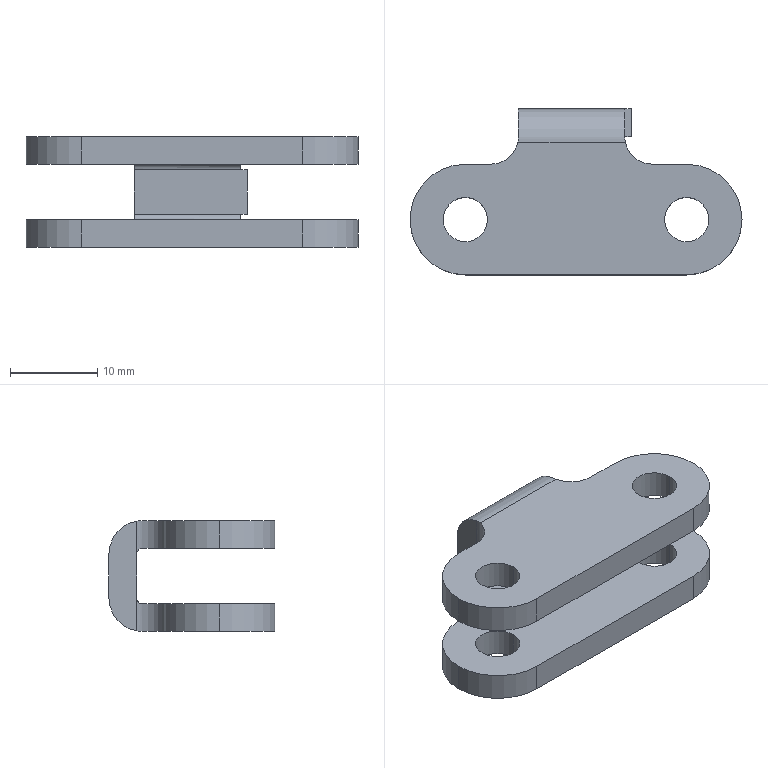Part | SolidWorks | features Cut 3, Fillet 3, Boss 1, Extrusion 1 | 1 solid | 42 faces | box 38.1 x 19.05 x 12.7 mm | volume 3299 mm3 | cylinder 24 | plane 18 | commonest cylinder face diameters 5.08 x8 12.7 x8 6.35 x4 1.27 x2 7.62 x2
STEP:
#1=CARTESIAN_POINT('',(0.9,0.,-0.5));
#2=VERTEX_POINT('',#1);
#3=CARTESIAN_POINT('',(1.1,0.,-0.5));
#4=VERTEX_POINT('',#3);
#5=CARTESIAN_POINT('',(1.,0.,-0.5));
#6=DIRECTION('',(0.,0.,1.));
#7=DIRECTION('',(1.,0.,0.));
#8=AXIS2_PLACEMENT_3D('',#5,#6,#7);
#9=CIRCLE('',#8,0.1);
#10=EDGE_CURVE('',#2,#4,#9,.T.);
#11=ORIENTED_EDGE('',*,*,#10,.F.);
#12=CARTESIAN_POINT('',(0.9,0.,-0.375));
#13=VERTEX_POINT('',#12);
#14=CARTESIAN_POINT('',(0.9,0.,-0.5));
#15=DIRECTION('',(0.,0.,1.));
#16=VECTOR('',#15,39.37);
#17=LINE('',#14,#16);
#18=EDGE_CURVE('',#2,#13,#17,.T.);
#19=ORIENTED_EDGE('',*,*,#18,.T.);
#20=CARTESIAN_POINT('',(1.1,0.,-0.375));
#21=VERTEX_POINT('',#20);
#22=CARTESIAN_POINT('',(1.,0.,-0.375));
#23=DIRECTION('',(0.,0.,1.));
#24=DIRECTION('',(0.,1.,0.));
#25=AXIS2_PLACEMENT_3D('',#22,#23,#24);
#26=CIRCLE('',#25,0.1);
#27=EDGE_CURVE('',#13,#21,#26,.T.);
#28=ORIENTED_EDGE('',*,*,#27,.T.);
#29=CARTESIAN_POINT('',(1.1,0.,-0.5));
#30=DIRECTION('',(0.,0.,1.));
#31=VECTOR('',#30,39.37);
#32=LINE('',#29,#31);
#33=EDGE_CURVE('',#4,#21,#32,.T.);
#34=ORIENTED_EDGE('',*,*,#33,.F.);
#35=EDGE_LOOP('',(#11,#19,#28,#34));
#36=FACE_OUTER_BOUND('',#35,.T.);
#37=CARTESIAN_POINT('',(1.,0.,-0.5));
#38=DIRECTION('',(0.,0.,1.));
#39=DIRECTION('',(1.,0.,0.));
#40=AXIS2_PLACEMENT_3D('',#37,#38,#39);
#41=CYLINDRICAL_SURFACE('',#40,0.1);
#42=ADVANCED_FACE('',(#36),#41,.F.);
#43=CARTESIAN_POINT('',(-0.1,0.,-0.5));
#44=VERTEX_POINT('',#43);
#45=CARTESIAN_POINT('',(0.1,0.,-0.5));
#46=VERTEX_POINT('',#45);
#47=CARTESIAN_POINT('',(0.,0.,-0.5));
#48=DIRECTION('',(0.,0.,1.));
#49=DIRECTION('',(1.,0.,0.));
#50=AXIS2_PLACEMENT_3D('',#47,#48,#49);
#51=CIRCLE('',#50,0.1);
#52=EDGE_CURVE('',#44,#46,#51,.T.);
#53=ORIENTED_EDGE('',*,*,#52,.F.);
#54=CARTESIAN_POINT('',(-0.1,0.,-0.375));
#55=VERTEX_POINT('',#54);
#56=CARTESIAN_POINT('',(-0.1,0.,-0.5));
#57=DIRECTION('',(0.,0.,1.));
#58=VECTOR('',#57,39.37);
#59=LINE('',#56,#58);
#60=EDGE_CURVE('',#44,#55,#59,.T.);
#61=ORIENTED_EDGE('',*,*,#60,.T.);
#62=CARTESIAN_POINT('',(0.1,0.,-0.375));
#63=VERTEX_POINT('',#62);
#64=CARTESIAN_POINT('',(0.,0.,-0.375));
#65=DIRECTION('',(0.,0.,1.));
#66=DIRECTION('',(0.,1.,0.));
#67=AXIS2_PLACEMENT_3D('',#64,#65,#66);
#68=CIRCLE('',#67,0.1);
#69=EDGE_CURVE('',#55,#63,#68,.T.);
#70=ORIENTED_EDGE('',*,*,#69,.T.);
#71=CARTESIAN_POINT('',(0.1,0.,-0.5));
#72=DIRECTION('',(0.,0.,1.));
#73=VECTOR('',#72,39.37);
#74=LINE('',#71,#73);
#75=EDGE_CURVE('',#46,#63,#74,.T.);
#76=ORIENTED_EDGE('',*,*,#75,.F.);
#77=EDGE_LOOP('',(#53,#61,#70,#76));
#78=FACE_OUTER_BOUND('',#77,.T.);
#79=CARTESIAN_POINT('',(0.,0.,-0.5));
#80=DIRECTION('',(0.,0.,1.));
#81=DIRECTION('',(1.,0.,0.));
#82=AXIS2_PLACEMENT_3D('',#79,#80,#81);
#83=CYLINDRICAL_SURFACE('',#82,0.1);
#84=ADVANCED_FACE('',(#78),#83,.F.);
#85=CARTESIAN_POINT('',(1.1,0.,-0.125));
#86=VERTEX_POINT('',#85);
#87=CARTESIAN_POINT('',(0.9,0.,-0.125));
#88=VERTEX_POINT('',#87);
#89=CARTESIAN_POINT('',(1.,0.,-0.125));
#90=DIRECTION('',(0.,0.,-1.));
#91=DIRECTION('',(0.,-1.,0.));
#92=AXIS2_PLACEMENT_3D('',#89,#90,#91);
#93=CIRCLE('',#92,0.1);
#94=EDGE_CURVE('',#86,#88,#93,.T.);
#95=ORIENTED_EDGE('',*,*,#94,.T.);
#96=CARTESIAN_POINT('',(0.9,0.,0.));
#97=VERTEX_POINT('',#96);
#98=CARTESIAN_POINT('',(0.9,0.,-0.5));
#99=DIRECTION('',(0.,0.,1.));
#100=VECTOR('',#99,39.37);
#101=LINE('',#98,#100);
#102=EDGE_CURVE('',#88,#97,#101,.T.);
#103=ORIENTED_EDGE('',*,*,#102,.T.);
#104=CARTESIAN_POINT('',(1.1,0.,0.));
#105=VERTEX_POINT('',#104);
#106=CARTESIAN_POINT('',(1.,0.,0.));
#107=DIRECTION('',(0.,0.,1.));
#108=DIRECTION('',(1.,0.,0.));
#109=AXIS2_PLACEMENT_3D('',#106,#107,#108);
#110=CIRCLE('',#109,0.1);
#111=EDGE_CURVE('',#97,#105,#110,.T.);
#112=ORIENTED_EDGE('',*,*,#111,.T.);
#113=CARTESIAN_POINT('',(1.1,0.,-0.5));
#114=DIRECTION('',(0.,0.,1.));
#115=VECTOR('',#114,39.37);
#116=LINE('',#113,#115);
#117=EDGE_CURVE('',#86,#105,#116,.T.);
#118=ORIENTED_EDGE('',*,*,#117,.F.);
#119=EDGE_LOOP('',(#95,#103,#112,#118));
#120=FACE_OUTER_BOUND('',#119,.T.);
#121=CARTESIAN_POINT('',(1.,0.,-0.5));
#122=DIRECTION('',(0.,0.,1.));
#123=DIRECTION('',(1.,0.,0.));
#124=AXIS2_PLACEMENT_3D('',#121,#122,#123);
#125=CYLINDRICAL_SURFACE('',#124,0.1);
#126=ADVANCED_FACE('',(#120),#125,.F.);
#127=CARTESIAN_POINT('',(0.1,0.,-0.125));
#128=VERTEX_POINT('',#127);
#129=CARTESIAN_POINT('',(-0.1,0.,-0.125));
#130=VERTEX_POINT('',#129);
#131=CARTESIAN_POINT('',(0.,0.,-0.125));
#132=DIRECTION('',(0.,0.,-1.));
#133=DIRECTION('',(0.,-1.,0.));
#134=AXIS2_PLACEMENT_3D('',#131,#132,#133);
#135=CIRCLE('',#134,0.1);
#136=EDGE_CURVE('',#128,#130,#135,.T.);
#137=ORIENTED_EDGE('',*,*,#136,.T.);
#138=CARTESIAN_POINT('',(-0.1,0.,0.));
#139=VERTEX_POINT('',#138);
#140=CARTESIAN_POINT('',(-0.1,0.,-0.5));
#141=DIRECTION('',(0.,0.,1.));
#142=VECTOR('',#141,39.37);
#143=LINE('',#140,#142);
#144=EDGE_CURVE('',#130,#139,#143,.T.);
#145=ORIENTED_EDGE('',*,*,#144,.T.);
#146=CARTESIAN_POINT('',(0.1,0.,0.));
#147=VERTEX_POINT('',#146);
#148=CARTESIAN_POINT('',(0.,0.,0.));
#149=DIRECTION('',(0.,0.,1.));
#150=DIRECTION('',(1.,0.,0.));
#151=AXIS2_PLACEMENT_3D('',#148,#149,#150);
#152=CIRCLE('',#151,0.1);
#153=EDGE_CURVE('',#139,#147,#152,.T.);
#154=ORIENTED_EDGE('',*,*,#153,.T.);
#155=CARTESIAN_POINT('',(0.1,0.,-0.5));
#156=DIRECTION('',(0.,0.,1.));
#157=VECTOR('',#156,39.37);
#158=LINE('',#155,#157);
#159=EDGE_CURVE('',#128,#147,#158,.T.);
#160=ORIENTED_EDGE('',*,*,#159,.F.);
#161=EDGE_LOOP('',(#137,#145,#154,#160));
#162=FACE_OUTER_BOUND('',#161,.T.);
#163=CARTESIAN_POINT('',(0.,0.,-0.5));
#164=DIRECTION('',(0.,0.,1.));
#165=DIRECTION('',(1.,0.,0.));
#166=AXIS2_PLACEMENT_3D('',#163,#164,#165);
#167=CYLINDRICAL_SURFACE('',#166,0.1);
#168=ADVANCED_FACE('',(#162),#167,.F.);
#169=CARTESIAN_POINT('',(0.72,0.5,-0.15));
#170=VERTEX_POINT('',#169);
#171=CARTESIAN_POINT('',(0.72,0.375,-0.15));
#172=VERTEX_POINT('',#171);
#173=CARTESIAN_POINT('',(0.72,0.5,-0.15));
#174=DIRECTION('',(0.,-1.,0.));
#175=VECTOR('',#174,39.37);
#176=LINE('',#173,#175);
#177=EDGE_CURVE('',#170,#172,#176,.T.);
#178=ORIENTED_EDGE('',*,*,#177,.F.);
#179=CARTESIAN_POINT('',(0.72,0.375,-0.002098));
#180=VERTEX_POINT('',#179);
#181=CARTESIAN_POINT('',(0.72,0.35,-0.15));
#182=DIRECTION('',(1.,0.,0.));
#183=DIRECTION('',(0.,-1.,0.));
#184=AXIS2_PLACEMENT_3D('',#181,#182,#183);
#185=CIRCLE('',#184,0.15);
#186=EDGE_CURVE('',#170,#180,#185,.T.);
#187=ORIENTED_EDGE('',*,*,#186,.T.);
#188=CARTESIAN_POINT('',(0.72,0.375,0.));
#189=DIRECTION('',(0.,0.,-1.));
#190=VECTOR('',#189,39.37);
#191=LINE('',#188,#190);
#192=EDGE_CURVE('',#180,#172,#191,.T.);
#193=ORIENTED_EDGE('',*,*,#192,.T.);
#194=EDGE_LOOP('',(#178,#187,#193));
#195=FACE_OUTER_BOUND('',#194,.T.);
#196=CARTESIAN_POINT('',(0.72,0.375,0.));
#197=DIRECTION('',(-1.,0.,0.));
#198=DIRECTION('',(0.,-1.,0.));
#199=AXIS2_PLACEMENT_3D('',#196,#197,#198);
#200=PLANE('',#199);
#201=ADVANCED_FACE('',(#195),#200,.F.);
#202=CARTESIAN_POINT('',(0.24,0.5,-0.15));
#203=VERTEX_POINT('',#202);
#204=CARTESIAN_POINT('',(0.24,0.5,-0.35));
#205=VERTEX_POINT('',#204);
#206=CARTESIAN_POINT('',(0.24,0.5,0.));
#207=DIRECTION('',(0.,0.,-1.));
#208=VECTOR('',#207,39.37);
#209=LINE('',#206,#208);
#210=EDGE_CURVE('',#203,#205,#209,.T.);
#211=ORIENTED_EDGE('',*,*,#210,.F.);
#212=CARTESIAN_POINT('',(0.72,0.5,-0.15));
#213=DIRECTION('',(1.,0.,0.));
#214=VECTOR('',#213,39.37);
#215=LINE('',#212,#214);
#216=EDGE_CURVE('',#203,#170,#215,.T.);
#217=ORIENTED_EDGE('',*,*,#216,.T.);
#218=CARTESIAN_POINT('',(0.75,0.5,-0.15));
#219=VERTEX_POINT('',#218);
#220=CARTESIAN_POINT('',(0.75,0.5,-0.15));
#221=DIRECTION('',(-1.,0.,0.));
#222=VECTOR('',#221,39.37);
#223=LINE('',#220,#222);
#224=EDGE_CURVE('',#219,#170,#223,.T.);
#225=ORIENTED_EDGE('',*,*,#224,.F.);
#226=CARTESIAN_POINT('',(0.75,0.5,-0.35));
#227=VERTEX_POINT('',#226);
#228=CARTESIAN_POINT('',(0.75,0.5,-0.15));
#229=DIRECTION('',(0.,0.,-1.));
#230=VECTOR('',#229,39.37);
#231=LINE('',#228,#230);
#232=EDGE_CURVE('',#219,#227,#231,.T.);
#233=ORIENTED_EDGE('',*,*,#232,.T.);
#234=CARTESIAN_POINT('',(0.72,0.5,-0.35));
#235=VERTEX_POINT('',#234);
#236=CARTESIAN_POINT('',(0.75,0.5,-0.35));
#237=DIRECTION('',(-1.,0.,0.));
#238=VECTOR('',#237,39.37);
#239=LINE('',#236,#238);
#240=EDGE_CURVE('',#227,#235,#239,.T.);
#241=ORIENTED_EDGE('',*,*,#240,.T.);
#242=CARTESIAN_POINT('',(1.25,0.5,-0.35));
#243=DIRECTION('',(-1.,0.,0.));
#244=VECTOR('',#243,39.37);
#245=LINE('',#242,#244);
#246=EDGE_CURVE('',#235,#205,#245,.T.);
#247=ORIENTED_EDGE('',*,*,#246,.T.);
#248=EDGE_LOOP('',(#211,#217,#225,#233,#241,#247));
#249=FACE_OUTER_BOUND('',#248,.T.);
#250=CARTESIAN_POINT('',(1.25,0.5,-0.5));
#251=DIRECTION('',(0.,1.,0.));
#252=DIRECTION('',(-1.,0.,0.));
#253=AXIS2_PLACEMENT_3D('',#250,#251,#252);
#254=PLANE('',#253);
#255=ADVANCED_FACE('',(#249),#254,.T.);
#256=CARTESIAN_POINT('',(0.,-0.25,-0.5));
#257=VERTEX_POINT('',#256);
#258=CARTESIAN_POINT('',(-0.25,0.,-0.5));
#259=VERTEX_POINT('',#258);
#260=CARTESIAN_POINT('',(0.,0.,-0.5));
#261=DIRECTION('',(0.,0.,-1.));
#262=DIRECTION('',(-1.,0.,0.));
#263=AXIS2_PLACEMENT_3D('',#260,#261,#262);
#264=CIRCLE('',#263,0.25);
#265=EDGE_CURVE('',#257,#259,#264,.T.);
#266=ORIENTED_EDGE('',*,*,#265,.T.);
#267=CARTESIAN_POINT('',(0.,0.25,-0.5));
#268=VERTEX_POINT('',#267);
#269=CARTESIAN_POINT('',(0.,0.,-0.5));
#270=DIRECTION('',(0.,0.,-1.));
#271=DIRECTION('',(-1.,0.,0.));
#272=AXIS2_PLACEMENT_3D('',#269,#270,#271);
#273=CIRCLE('',#272,0.25);
#274=EDGE_CURVE('',#259,#268,#273,.T.);
#275=ORIENTED_EDGE('',*,*,#274,.T.);
#276=CARTESIAN_POINT('',(0.115,0.25,-0.5));
#277=VERTEX_POINT('',#276);
#278=CARTESIAN_POINT('',(-0.25,0.25,-0.5));
#279=DIRECTION('',(1.,0.,0.));
#280=VECTOR('',#279,39.37);
#281=LINE('',#278,#280);
#282=EDGE_CURVE('',#268,#277,#281,.T.);
#283=ORIENTED_EDGE('',*,*,#282,.T.);
#284=CARTESIAN_POINT('',(0.2375,0.35,-0.5));
#285=VERTEX_POINT('',#284);
#286=CARTESIAN_POINT('',(0.115,0.375,-0.5));
#287=DIRECTION('',(0.,0.,1.));
#288=DIRECTION('',(-1.,0.,0.));
#289=AXIS2_PLACEMENT_3D('',#286,#287,#288);
#290=CIRCLE('',#289,0.125);
#291=EDGE_CURVE('',#277,#285,#290,.T.);
#292=ORIENTED_EDGE('',*,*,#291,.T.);
#293=CARTESIAN_POINT('',(0.7225,0.35,-0.5));
#294=VERTEX_POINT('',#293);
#295=CARTESIAN_POINT('',(-0.25,0.35,-0.5));
#296=DIRECTION('',(1.,0.,0.));
#297=VECTOR('',#296,39.37);
#298=LINE('',#295,#297);
#299=EDGE_CURVE('',#285,#294,#298,.T.);
#300=ORIENTED_EDGE('',*,*,#299,.T.);
#301=CARTESIAN_POINT('',(0.845,0.25,-0.5));
#302=VERTEX_POINT('',#301);
#303=CARTESIAN_POINT('',(0.845,0.375,-0.5));
#304=DIRECTION('',(0.,0.,-1.));
#305=DIRECTION('',(-1.,0.,0.));
#306=AXIS2_PLACEMENT_3D('',#303,#304,#305);
#307=CIRCLE('',#306,0.125);
#308=EDGE_CURVE('',#302,#294,#307,.T.);
#309=ORIENTED_EDGE('',*,*,#308,.F.);
#310=CARTESIAN_POINT('',(1.,0.25,-0.5));
#311=VERTEX_POINT('',#310);
#312=CARTESIAN_POINT('',(-0.25,0.25,-0.5));
#313=DIRECTION('',(-1.,0.,0.));
#314=VECTOR('',#313,39.37);
#315=LINE('',#312,#314);
#316=EDGE_CURVE('',#311,#302,#315,.T.);
#317=ORIENTED_EDGE('',*,*,#316,.F.);
#318=CARTESIAN_POINT('',(1.25,0.,-0.5));
#319=VERTEX_POINT('',#318);
#320=CARTESIAN_POINT('',(1.,0.,-0.5));
#321=DIRECTION('',(0.,0.,-1.));
#322=DIRECTION('',(-1.,0.,0.));
#323=AXIS2_PLACEMENT_3D('',#320,#321,#322);
#324=CIRCLE('',#323,0.25);
#325=EDGE_CURVE('',#311,#319,#324,.T.);
#326=ORIENTED_EDGE('',*,*,#325,.T.);
#327=CARTESIAN_POINT('',(1.,-0.25,-0.5));
#328=VERTEX_POINT('',#327);
#329=CARTESIAN_POINT('',(1.,0.,-0.5));
#330=DIRECTION('',(0.,0.,-1.));
#331=DIRECTION('',(-1.,0.,0.));
#332=AXIS2_PLACEMENT_3D('',#329,#330,#331);
#333=CIRCLE('',#332,0.25);
#334=EDGE_CURVE('',#319,#328,#333,.T.);
#335=ORIENTED_EDGE('',*,*,#334,.T.);
#336=CARTESIAN_POINT('',(-0.25,-0.25,-0.5));
#337=DIRECTION('',(1.,0.,0.));
#338=VECTOR('',#337,39.37);
#339=LINE('',#336,#338);
#340=EDGE_CURVE('',#257,#328,#339,.T.);
#341=ORIENTED_EDGE('',*,*,#340,.F.);
#342=EDGE_LOOP('',(#266,#275,#283,#292,#300,#309,#317,#326,#335,#341));
#343=FACE_OUTER_BOUND('',#342,.T.);
#344=CARTESIAN_POINT('',(0.,0.,-0.5));
#345=DIRECTION('',(0.,0.,1.));
#346=DIRECTION('',(1.,0.,0.));
#347=AXIS2_PLACEMENT_3D('',#344,#345,#346);
#348=CIRCLE('',#347,0.1);
#349=EDGE_CURVE('',#46,#44,#348,.T.);
#350=ORIENTED_EDGE('',*,*,#349,.T.);
#351=ORIENTED_EDGE('',*,*,#52,.T.);
#352=EDGE_LOOP('',(#350,#351));
#353=FACE_BOUND('',#352,.T.);
#354=CARTESIAN_POINT('',(1.,0.,-0.5));
#355=DIRECTION('',(0.,0.,1.));
#356=DIRECTION('',(1.,0.,0.));
#357=AXIS2_PLACEMENT_3D('',#354,#355,#356);
#358=CIRCLE('',#357,0.1);
#359=EDGE_CURVE('',#4,#2,#358,.T.);
#360=ORIENTED_EDGE('',*,*,#359,.T.);
#361=ORIENTED_EDGE('',*,*,#10,.T.);
#362=EDGE_LOOP('',(#360,#361));
#363=FACE_BOUND('',#362,.T.);
#364=CARTESIAN_POINT('',(-0.25,-0.25,-0.5));
#365=DIRECTION('',(0.,0.,-1.));
#366=DIRECTION('',(-1.,0.,0.));
#367=AXIS2_PLACEMENT_3D('',#364,#365,#366);
#368=PLANE('',#367);
#369=ADVANCED_FACE('',(#343,#353,#363),#368,.T.);
#370=CARTESIAN_POINT('',(0.,0.,0.));
#371=DIRECTION('',(0.,0.,1.));
#372=DIRECTION('',(1.,0.,0.));
#373=AXIS2_PLACEMENT_3D('',#370,#371,#372);
#374=CIRCLE('',#373,0.1);
#375=EDGE_CURVE('',#147,#139,#374,.T.);
#376=ORIENTED_EDGE('',*,*,#375,.F.);
#377=ORIENTED_EDGE('',*,*,#153,.F.);
#378=EDGE_LOOP('',(#376,#377));
#379=FACE_BOUND('',#378,.T.);
#380=CARTESIAN_POINT('',(1.,0.,0.));
#381=DIRECTION('',(0.,0.,1.));
#382=DIRECTION('',(1.,0.,0.));
#383=AXIS2_PLACEMENT_3D('',#380,#381,#382);
#384=CIRCLE('',#383,0.1);
#385=EDGE_CURVE('',#105,#97,#384,.T.);
#386=ORIENTED_EDGE('',*,*,#385,.F.);
#387=ORIENTED_EDGE('',*,*,#111,.F.);
#388=EDGE_LOOP('',(#386,#387));
#389=FACE_BOUND('',#388,.T.);
#390=CARTESIAN_POINT('',(0.,0.25,0.));
#391=VERTEX_POINT('',#390);
#392=CARTESIAN_POINT('',(0.115,0.25,0.));
#393=VERTEX_POINT('',#392);
#394=CARTESIAN_POINT('',(-0.25,0.25,0.));
#395=DIRECTION('',(1.,0.,0.));
#396=VECTOR('',#395,39.37);
#397=LINE('',#394,#396);
#398=EDGE_CURVE('',#391,#393,#397,.T.);
#399=ORIENTED_EDGE('',*,*,#398,.F.);
#400=CARTESIAN_POINT('',(-0.25,0.,0.));
#401=VERTEX_POINT('',#400);
#402=CARTESIAN_POINT('',(0.,0.,0.));
#403=DIRECTION('',(0.,0.,1.));
#404=DIRECTION('',(-1.,0.,0.));
#405=AXIS2_PLACEMENT_3D('',#402,#403,#404);
#406=CIRCLE('',#405,0.25);
#407=EDGE_CURVE('',#391,#401,#406,.T.);
#408=ORIENTED_EDGE('',*,*,#407,.T.);
#409=CARTESIAN_POINT('',(0.,-0.25,0.));
#410=VERTEX_POINT('',#409);
#411=CARTESIAN_POINT('',(0.,0.,0.));
#412=DIRECTION('',(0.,0.,1.));
#413=DIRECTION('',(-1.,0.,0.));
#414=AXIS2_PLACEMENT_3D('',#411,#412,#413);
#415=CIRCLE('',#414,0.25);
#416=EDGE_CURVE('',#401,#410,#415,.T.);
#417=ORIENTED_EDGE('',*,*,#416,.T.);
#418=CARTESIAN_POINT('',(1.,-0.25,0.));
#419=VERTEX_POINT('',#418);
#420=CARTESIAN_POINT('',(-0.25,-0.25,0.));
#421=DIRECTION('',(1.,0.,0.));
#422=VECTOR('',#421,39.37);
#423=LINE('',#420,#422);
#424=EDGE_CURVE('',#410,#419,#423,.T.);
#425=ORIENTED_EDGE('',*,*,#424,.T.);
#426=CARTESIAN_POINT('',(1.25,0.,0.));
#427=VERTEX_POINT('',#426);
#428=CARTESIAN_POINT('',(1.,0.,0.));
#429=DIRECTION('',(0.,0.,1.));
#430=DIRECTION('',(-1.,0.,0.));
#431=AXIS2_PLACEMENT_3D('',#428,#429,#430);
#432=CIRCLE('',#431,0.25);
#433=EDGE_CURVE('',#419,#427,#432,.T.);
#434=ORIENTED_EDGE('',*,*,#433,.T.);
#435=CARTESIAN_POINT('',(1.,0.25,0.));
#436=VERTEX_POINT('',#435);
#437=CARTESIAN_POINT('',(1.,0.,0.));
#438=DIRECTION('',(0.,0.,1.));
#439=DIRECTION('',(-1.,0.,0.));
#440=AXIS2_PLACEMENT_3D('',#437,#438,#439);
#441=CIRCLE('',#440,0.25);
#442=EDGE_CURVE('',#427,#436,#441,.T.);
#443=ORIENTED_EDGE('',*,*,#442,.T.);
#444=CARTESIAN_POINT('',(0.845,0.25,0.));
#445=VERTEX_POINT('',#444);
#446=CARTESIAN_POINT('',(1.25,0.25,0.));
#447=DIRECTION('',(-1.,0.,0.));
#448=VECTOR('',#447,39.37);
#449=LINE('',#446,#448);
#450=EDGE_CURVE('',#436,#445,#449,.T.);
#451=ORIENTED_EDGE('',*,*,#450,.T.);
#452=CARTESIAN_POINT('',(0.7225,0.35,0.));
#453=VERTEX_POINT('',#452);
#454=CARTESIAN_POINT('',(0.845,0.375,0.));
#455=DIRECTION('',(0.,0.,-1.));
#456=DIRECTION('',(-1.,0.,0.));
#457=AXIS2_PLACEMENT_3D('',#454,#455,#456);
#458=CIRCLE('',#457,0.125);
#459=EDGE_CURVE('',#445,#453,#458,.T.);
#460=ORIENTED_EDGE('',*,*,#459,.T.);
#461=CARTESIAN_POINT('',(0.2375,0.35,0.));
#462=VERTEX_POINT('',#461);
#463=CARTESIAN_POINT('',(0.24,0.35,0.));
#464=DIRECTION('',(-1.,0.,0.));
#465=VECTOR('',#464,39.37);
#466=LINE('',#463,#465);
#467=EDGE_CURVE('',#453,#462,#466,.T.);
#468=ORIENTED_EDGE('',*,*,#467,.T.);
#469=CARTESIAN_POINT('',(0.115,0.375,0.));
#470=DIRECTION('',(0.,0.,1.));
#471=DIRECTION('',(1.,0.,0.));
#472=AXIS2_PLACEMENT_3D('',#469,#470,#471);
#473=CIRCLE('',#472,0.125);
#474=EDGE_CURVE('',#393,#462,#473,.T.);
#475=ORIENTED_EDGE('',*,*,#474,.F.);
#476=EDGE_LOOP('',(#399,#408,#417,#425,#434,#443,#451,#460,#468,#475));
#477=FACE_OUTER_BOUND('',#476,.T.);
#478=CARTESIAN_POINT('',(-0.25,-0.25,0.));
#479=DIRECTION('',(0.,0.,-1.));
#480=DIRECTION('',(-1.,0.,0.));
#481=AXIS2_PLACEMENT_3D('',#478,#479,#480);
#482=PLANE('',#481);
#483=ADVANCED_FACE('',(#379,#389,#477),#482,.F.);
#484=CARTESIAN_POINT('',(0.24,0.375,-0.35));
#485=VERTEX_POINT('',#484);
#486=CARTESIAN_POINT('',(0.72,0.375,-0.35));
#487=VERTEX_POINT('',#486);
#488=CARTESIAN_POINT('',(0.72,0.375,-0.35));
#489=DIRECTION('',(1.,0.,0.));
#490=VECTOR('',#489,39.37);
#491=LINE('',#488,#490);
#492=EDGE_CURVE('',#485,#487,#491,.T.);
#493=ORIENTED_EDGE('',*,*,#492,.T.);
#494=CARTESIAN_POINT('',(0.75,0.375,-0.35));
#495=VERTEX_POINT('',#494);
#496=CARTESIAN_POINT('',(0.75,0.375,-0.35));
#497=DIRECTION('',(-1.,0.,0.));
#498=VECTOR('',#497,39.37);
#499=LINE('',#496,#498);
#500=EDGE_CURVE('',#495,#487,#499,.T.);
#501=ORIENTED_EDGE('',*,*,#500,.F.);
#502=CARTESIAN_POINT('',(0.75,0.375,-0.15));
#503=VERTEX_POINT('',#502);
#504=CARTESIAN_POINT('',(0.75,0.375,-0.15));
#505=DIRECTION('',(0.,0.,-1.));
#506=VECTOR('',#505,39.37);
#507=LINE('',#504,#506);
#508=EDGE_CURVE('',#503,#495,#507,.T.);
#509=ORIENTED_EDGE('',*,*,#508,.F.);
#510=CARTESIAN_POINT('',(0.75,0.375,-0.15));
#511=DIRECTION('',(-1.,0.,0.));
#512=VECTOR('',#511,39.37);
#513=LINE('',#510,#512);
#514=EDGE_CURVE('',#503,#172,#513,.T.);
#515=ORIENTED_EDGE('',*,*,#514,.T.);
#516=CARTESIAN_POINT('',(0.24,0.375,-0.15));
#517=VERTEX_POINT('',#516);
#518=CARTESIAN_POINT('',(0.24,0.375,-0.15));
#519=DIRECTION('',(-1.,0.,0.));
#520=VECTOR('',#519,39.37);
#521=LINE('',#518,#520);
#522=EDGE_CURVE('',#172,#517,#521,.T.);
#523=ORIENTED_EDGE('',*,*,#522,.T.);
#524=CARTESIAN_POINT('',(0.24,0.375,0.));
#525=DIRECTION('',(0.,0.,-1.));
#526=VECTOR('',#525,39.37);
#527=LINE('',#524,#526);
#528=EDGE_CURVE('',#517,#485,#527,.T.);
#529=ORIENTED_EDGE('',*,*,#528,.T.);
#530=EDGE_LOOP('',(#493,#501,#509,#515,#523,#529));
#531=FACE_OUTER_BOUND('',#530,.T.);
#532=CARTESIAN_POINT('',(1.25,0.375,-0.125));
#533=DIRECTION('',(0.,1.,0.));
#534=DIRECTION('',(0.,0.,1.));
#535=AXIS2_PLACEMENT_3D('',#532,#533,#534);
#536=PLANE('',#535);
#537=ADVANCED_FACE('',(#531),#536,.F.);
#538=ORIENTED_EDGE('',*,*,#94,.F.);
#539=CARTESIAN_POINT('',(1.,0.,-0.125));
#540=DIRECTION('',(0.,0.,-1.));
#541=DIRECTION('',(0.,-1.,0.));
#542=AXIS2_PLACEMENT_3D('',#539,#540,#541);
#543=CIRCLE('',#542,0.1);
#544=EDGE_CURVE('',#88,#86,#543,.T.);
#545=ORIENTED_EDGE('',*,*,#544,.F.);
#546=EDGE_LOOP('',(#538,#545));
#547=FACE_BOUND('',#546,.T.);
#548=ORIENTED_EDGE('',*,*,#136,.F.);
#549=CARTESIAN_POINT('',(0.,0.,-0.125));
#550=DIRECTION('',(0.,0.,-1.));
#551=DIRECTION('',(0.,-1.,0.));
#552=AXIS2_PLACEMENT_3D('',#549,#550,#551);
#553=CIRCLE('',#552,0.1);
#554=EDGE_CURVE('',#130,#128,#553,.T.);
#555=ORIENTED_EDGE('',*,*,#554,.F.);
#556=EDGE_LOOP('',(#548,#555));
#557=FACE_BOUND('',#556,.T.);
#558=CARTESIAN_POINT('',(0.,-0.25,-0.125));
#559=VERTEX_POINT('',#558);
#560=CARTESIAN_POINT('',(-0.25,0.,-0.125));
#561=VERTEX_POINT('',#560);
#562=CARTESIAN_POINT('',(0.,0.,-0.125));
#563=DIRECTION('',(0.,0.,-1.));
#564=DIRECTION('',(0.,-1.,0.));
#565=AXIS2_PLACEMENT_3D('',#562,#563,#564);
#566=CIRCLE('',#565,0.25);
#567=EDGE_CURVE('',#559,#561,#566,.T.);
#568=ORIENTED_EDGE('',*,*,#567,.T.);
#569=CARTESIAN_POINT('',(0.,0.25,-0.125));
#570=VERTEX_POINT('',#569);
#571=CARTESIAN_POINT('',(0.,0.,-0.125));
#572=DIRECTION('',(0.,0.,-1.));
#573=DIRECTION('',(0.,-1.,0.));
#574=AXIS2_PLACEMENT_3D('',#571,#572,#573);
#575=CIRCLE('',#574,0.25);
#576=EDGE_CURVE('',#561,#570,#575,.T.);
#577=ORIENTED_EDGE('',*,*,#576,.T.);
#578=CARTESIAN_POINT('',(0.115,0.25,-0.125));
#579=VERTEX_POINT('',#578);
#580=CARTESIAN_POINT('',(1.25,0.25,-0.125));
#581=DIRECTION('',(-1.,0.,0.));
#582=VECTOR('',#581,39.37);
#583=LINE('',#580,#582);
#584=EDGE_CURVE('',#579,#570,#583,.T.);
#585=ORIENTED_EDGE('',*,*,#584,.F.);
#586=CARTESIAN_POINT('',(0.2375,0.35,-0.125));
#587=VERTEX_POINT('',#586);
#588=CARTESIAN_POINT('',(0.115,0.375,-0.125));
#589=DIRECTION('',(0.,0.,-1.));
#590=DIRECTION('',(0.,-1.,0.));
#591=AXIS2_PLACEMENT_3D('',#588,#589,#590);
#592=CIRCLE('',#591,0.125);
#593=EDGE_CURVE('',#587,#579,#592,.T.);
#594=ORIENTED_EDGE('',*,*,#593,.F.);
#595=CARTESIAN_POINT('',(0.7225,0.35,-0.125));
#596=VERTEX_POINT('',#595);
#597=CARTESIAN_POINT('',(0.72,0.35,-0.125));
#598=DIRECTION('',(1.,0.,0.));
#599=VECTOR('',#598,39.37);
#600=LINE('',#597,#599);
#601=EDGE_CURVE('',#587,#596,#600,.T.);
#602=ORIENTED_EDGE('',*,*,#601,.T.);
#603=CARTESIAN_POINT('',(0.845,0.25,-0.125));
#604=VERTEX_POINT('',#603);
#605=CARTESIAN_POINT('',(0.845,0.375,-0.125));
#606=DIRECTION('',(0.,0.,1.));
#607=DIRECTION('',(0.,-1.,0.));
#608=AXIS2_PLACEMENT_3D('',#605,#606,#607);
#609=CIRCLE('',#608,0.125);
#610=EDGE_CURVE('',#596,#604,#609,.T.);
#611=ORIENTED_EDGE('',*,*,#610,.T.);
#612=CARTESIAN_POINT('',(1.,0.25,-0.125));
#613=VERTEX_POINT('',#612);
#614=CARTESIAN_POINT('',(1.25,0.25,-0.125));
#615=DIRECTION('',(1.,0.,0.));
#616=VECTOR('',#615,39.37);
#617=LINE('',#614,#616);
#618=EDGE_CURVE('',#604,#613,#617,.T.);
#619=ORIENTED_EDGE('',*,*,#618,.T.);
#620=CARTESIAN_POINT('',(1.25,0.,-0.125));
#621=VERTEX_POINT('',#620);
#622=CARTESIAN_POINT('',(1.,0.,-0.125));
#623=DIRECTION('',(0.,0.,-1.));
#624=DIRECTION('',(0.,-1.,0.));
#625=AXIS2_PLACEMENT_3D('',#622,#623,#624);
#626=CIRCLE('',#625,0.25);
#627=EDGE_CURVE('',#613,#621,#626,.T.);
#628=ORIENTED_EDGE('',*,*,#627,.T.);
#629=CARTESIAN_POINT('',(1.,-0.25,-0.125));
#630=VERTEX_POINT('',#629);
#631=CARTESIAN_POINT('',(1.,0.,-0.125));
#632=DIRECTION('',(0.,0.,-1.));
#633=DIRECTION('',(0.,-1.,0.));
#634=AXIS2_PLACEMENT_3D('',#631,#632,#633);
#635=CIRCLE('',#634,0.25);
#636=EDGE_CURVE('',#621,#630,#635,.T.);
#637=ORIENTED_EDGE('',*,*,#636,.T.);
#638=CARTESIAN_POINT('',(1.25,-0.25,-0.125));
#639=DIRECTION('',(-1.,0.,0.));
#640=VECTOR('',#639,39.37);
#641=LINE('',#638,#640);
#642=EDGE_CURVE('',#630,#559,#641,.T.);
#643=ORIENTED_EDGE('',*,*,#642,.T.);
#644=EDGE_LOOP('',(#568,#577,#585,#594,#602,#611,#619,#628,#637,#643));
#645=FACE_OUTER_BOUND('',#644,.T.);
#646=CARTESIAN_POINT('',(1.25,-0.25,-0.125));
#647=DIRECTION('',(0.,0.,1.));
#648=DIRECTION('',(0.,-1.,0.));
#649=AXIS2_PLACEMENT_3D('',#646,#647,#648);
#650=PLANE('',#649);
#651=ADVANCED_FACE('',(#547,#557,#645),#650,.F.);
#652=CARTESIAN_POINT('',(1.,0.,-0.375));
#653=DIRECTION('',(0.,0.,1.));
#654=DIRECTION('',(0.,1.,0.));
#655=AXIS2_PLACEMENT_3D('',#652,#653,#654);
#656=CIRCLE('',#655,0.1);
#657=EDGE_CURVE('',#21,#13,#656,.T.);
#658=ORIENTED_EDGE('',*,*,#657,.F.);
#659=ORIENTED_EDGE('',*,*,#27,.F.);
#660=EDGE_LOOP('',(#658,#659));
#661=FACE_BOUND('',#660,.T.);
#662=CARTESIAN_POINT('',(0.,0.,-0.375));
#663=DIRECTION('',(0.,0.,1.));
#664=DIRECTION('',(0.,1.,0.));
#665=AXIS2_PLACEMENT_3D('',#662,#663,#664);
#666=CIRCLE('',#665,0.1);
#667=EDGE_CURVE('',#63,#55,#666,.T.);
#668=ORIENTED_EDGE('',*,*,#667,.F.);
#669=ORIENTED_EDGE('',*,*,#69,.F.);
#670=EDGE_LOOP('',(#668,#669));
#671=FACE_BOUND('',#670,.T.);
#672=CARTESIAN_POINT('',(0.,0.25,-0.375));
#673=VERTEX_POINT('',#672);
#674=CARTESIAN_POINT('',(0.115,0.25,-0.375));
#675=VERTEX_POINT('',#674);
#676=CARTESIAN_POINT('',(1.25,0.25,-0.375));
#677=DIRECTION('',(1.,0.,0.));
#678=VECTOR('',#677,39.37);
#679=LINE('',#676,#678);
#680=EDGE_CURVE('',#673,#675,#679,.T.);
#681=ORIENTED_EDGE('',*,*,#680,.F.);
#682=CARTESIAN_POINT('',(-0.25,0.,-0.375));
#683=VERTEX_POINT('',#682);
#684=CARTESIAN_POINT('',(0.,0.,-0.375));
#685=DIRECTION('',(0.,0.,1.));
#686=DIRECTION('',(0.,1.,0.));
#687=AXIS2_PLACEMENT_3D('',#684,#685,#686);
#688=CIRCLE('',#687,0.25);
#689=EDGE_CURVE('',#673,#683,#688,.T.);
#690=ORIENTED_EDGE('',*,*,#689,.T.);
#691=CARTESIAN_POINT('',(0.,-0.25,-0.375));
#692=VERTEX_POINT('',#691);
#693=CARTESIAN_POINT('',(0.,0.,-0.375));
#694=DIRECTION('',(0.,0.,1.));
#695=DIRECTION('',(0.,1.,0.));
#696=AXIS2_PLACEMENT_3D('',#693,#694,#695);
#697=CIRCLE('',#696,0.25);
#698=EDGE_CURVE('',#683,#692,#697,.T.);
#699=ORIENTED_EDGE('',*,*,#698,.T.);
#700=CARTESIAN_POINT('',(1.,-0.25,-0.375));
#701=VERTEX_POINT('',#700);
#702=CARTESIAN_POINT('',(1.25,-0.25,-0.375));
#703=DIRECTION('',(-1.,0.,0.));
#704=VECTOR('',#703,39.37);
#705=LINE('',#702,#704);
#706=EDGE_CURVE('',#701,#692,#705,.T.);
#707=ORIENTED_EDGE('',*,*,#706,.F.);
#708=CARTESIAN_POINT('',(1.25,0.,-0.375));
#709=VERTEX_POINT('',#708);
#710=CARTESIAN_POINT('',(1.,0.,-0.375));
#711=DIRECTION('',(0.,0.,1.));
#712=DIRECTION('',(0.,1.,0.));
#713=AXIS2_PLACEMENT_3D('',#710,#711,#712);
#714=CIRCLE('',#713,0.25);
#715=EDGE_CURVE('',#701,#709,#714,.T.);
#716=ORIENTED_EDGE('',*,*,#715,.T.);
#717=CARTESIAN_POINT('',(1.,0.25,-0.375));
#718=VERTEX_POINT('',#717);
#719=CARTESIAN_POINT('',(1.,0.,-0.375));
#720=DIRECTION('',(0.,0.,1.));
#721=DIRECTION('',(0.,1.,0.));
#722=AXIS2_PLACEMENT_3D('',#719,#720,#721);
#723=CIRCLE('',#722,0.25);
#724=EDGE_CURVE('',#709,#718,#723,.T.);
#725=ORIENTED_EDGE('',*,*,#724,.T.);
#726=CARTESIAN_POINT('',(0.845,0.25,-0.375));
#727=VERTEX_POINT('',#726);
#728=CARTESIAN_POINT('',(1.25,0.25,-0.375));
#729=DIRECTION('',(-1.,0.,0.));
#730=VECTOR('',#729,39.37);
#731=LINE('',#728,#730);
#732=EDGE_CURVE('',#718,#727,#731,.T.);
#733=ORIENTED_EDGE('',*,*,#732,.T.);
#734=CARTESIAN_POINT('',(0.7225,0.35,-0.375));
#735=VERTEX_POINT('',#734);
#736=CARTESIAN_POINT('',(0.845,0.375,-0.375));
#737=DIRECTION('',(0.,0.,-1.));
#738=DIRECTION('',(0.,1.,0.));
#739=AXIS2_PLACEMENT_3D('',#736,#737,#738);
#740=CIRCLE('',#739,0.125);
#741=EDGE_CURVE('',#727,#735,#740,.T.);
#742=ORIENTED_EDGE('',*,*,#741,.T.);
#743=CARTESIAN_POINT('',(0.2375,0.35,-0.375));
#744=VERTEX_POINT('',#743);
#745=CARTESIAN_POINT('',(0.24,0.35,-0.375));
#746=DIRECTION('',(-1.,0.,0.));
#747=VECTOR('',#746,39.37);
#748=LINE('',#745,#747);
#749=EDGE_CURVE('',#735,#744,#748,.T.);
#750=ORIENTED_EDGE('',*,*,#749,.T.);
#751=CARTESIAN_POINT('',(0.115,0.375,-0.375));
#752=DIRECTION('',(0.,0.,1.));
#753=DIRECTION('',(0.,1.,0.));
#754=AXIS2_PLACEMENT_3D('',#751,#752,#753);
#755=CIRCLE('',#754,0.125);
#756=EDGE_CURVE('',#675,#744,#755,.T.);
#757=ORIENTED_EDGE('',*,*,#756,.F.);
#758=EDGE_LOOP('',(#681,#690,#699,#707,#716,#725,#733,#742,#750,#757));
#759=FACE_OUTER_BOUND('',#758,.T.);
#760=CARTESIAN_POINT('',(1.25,0.375,-0.375));
#761=DIRECTION('',(0.,0.,-1.));
#762=DIRECTION('',(0.,1.,0.));
#763=AXIS2_PLACEMENT_3D('',#760,#761,#762);
#764=PLANE('',#763);
#765=ADVANCED_FACE('',(#661,#671,#759),#764,.F.);
#766=ORIENTED_EDGE('',*,*,#424,.F.);
#767=CARTESIAN_POINT('',(0.,-0.25,-0.125));
#768=DIRECTION('',(0.,0.,-1.));
#769=VECTOR('',#768,39.37);
#770=LINE('',#767,#769);
#771=EDGE_CURVE('',#410,#559,#770,.T.);
#772=ORIENTED_EDGE('',*,*,#771,.T.);
#773=ORIENTED_EDGE('',*,*,#642,.F.);
#774=CARTESIAN_POINT('',(1.,-0.25,0.));
#775=DIRECTION('',(0.,0.,1.));
#776=VECTOR('',#775,39.37);
#777=LINE('',#774,#776);
#778=EDGE_CURVE('',#630,#419,#777,.T.);
#779=ORIENTED_EDGE('',*,*,#778,.T.);
#780=EDGE_LOOP('',(#766,#772,#773,#779));
#781=FACE_OUTER_BOUND('',#780,.T.);
#782=CARTESIAN_POINT('',(-0.25,-0.25,-0.5));
#783=DIRECTION('',(0.,-1.,0.));
#784=DIRECTION('',(0.,0.,-1.));
#785=AXIS2_PLACEMENT_3D('',#782,#783,#784);
#786=PLANE('',#785);
#787=ADVANCED_FACE('',(#781),#786,.T.);
#788=ORIENTED_EDGE('',*,*,#144,.F.);
#789=ORIENTED_EDGE('',*,*,#554,.T.);
#790=ORIENTED_EDGE('',*,*,#159,.T.);
#791=ORIENTED_EDGE('',*,*,#375,.T.);
#792=EDGE_LOOP('',(#788,#789,#790,#791));
#793=FACE_OUTER_BOUND('',#792,.T.);
#794=CARTESIAN_POINT('',(0.,0.,-0.5));
#795=DIRECTION('',(0.,0.,1.));
#796=DIRECTION('',(1.,0.,0.));
#797=AXIS2_PLACEMENT_3D('',#794,#795,#796);
#798=CYLINDRICAL_SURFACE('',#797,0.1);
#799=ADVANCED_FACE('',(#793),#798,.F.);
#800=ORIENTED_EDGE('',*,*,#102,.F.);
#801=ORIENTED_EDGE('',*,*,#544,.T.);
#802=ORIENTED_EDGE('',*,*,#117,.T.);
#803=ORIENTED_EDGE('',*,*,#385,.T.);
#804=EDGE_LOOP('',(#800,#801,#802,#803));
#805=FACE_OUTER_BOUND('',#804,.T.);
#806=CARTESIAN_POINT('',(1.,0.,-0.5));
#807=DIRECTION('',(0.,0.,1.));
#808=DIRECTION('',(1.,0.,0.));
#809=AXIS2_PLACEMENT_3D('',#806,#807,#808);
#810=CYLINDRICAL_SURFACE('',#809,0.1);
#811=ADVANCED_FACE('',(#805),#810,.F.);
#812=ORIENTED_EDGE('',*,*,#706,.T.);
#813=CARTESIAN_POINT('',(0.,-0.25,-0.5));
#814=DIRECTION('',(0.,0.,-1.));
#815=VECTOR('',#814,39.37);
#816=LINE('',#813,#815);
#817=EDGE_CURVE('',#692,#257,#816,.T.);
#818=ORIENTED_EDGE('',*,*,#817,.T.);
#819=ORIENTED_EDGE('',*,*,#340,.T.);
#820=CARTESIAN_POINT('',(1.,-0.25,-0.375));
#821=DIRECTION('',(0.,0.,1.));
#822=VECTOR('',#821,39.37);
#823=LINE('',#820,#822);
#824=EDGE_CURVE('',#328,#701,#823,.T.);
#825=ORIENTED_EDGE('',*,*,#824,.T.);
#826=EDGE_LOOP('',(#812,#818,#819,#825));
#827=FACE_OUTER_BOUND('',#826,.T.);
#828=CARTESIAN_POINT('',(-0.25,-0.25,-0.5));
#829=DIRECTION('',(0.,-1.,0.));
#830=DIRECTION('',(0.,0.,-1.));
#831=AXIS2_PLACEMENT_3D('',#828,#829,#830);
#832=PLANE('',#831);
#833=ADVANCED_FACE('',(#827),#832,.T.);
#834=ORIENTED_EDGE('',*,*,#60,.F.);
#835=ORIENTED_EDGE('',*,*,#349,.F.);
#836=ORIENTED_EDGE('',*,*,#75,.T.);
#837=ORIENTED_EDGE('',*,*,#667,.T.);
#838=EDGE_LOOP('',(#834,#835,#836,#837));
#839=FACE_OUTER_BOUND('',#838,.T.);
#840=CARTESIAN_POINT('',(0.,0.,-0.5));
#841=DIRECTION('',(0.,0.,1.));
#842=DIRECTION('',(1.,0.,0.));
#843=AXIS2_PLACEMENT_3D('',#840,#841,#842);
#844=CYLINDRICAL_SURFACE('',#843,0.1);
#845=ADVANCED_FACE('',(#839),#844,.F.);
#846=ORIENTED_EDGE('',*,*,#18,.F.);
#847=ORIENTED_EDGE('',*,*,#359,.F.);
#848=ORIENTED_EDGE('',*,*,#33,.T.);
#849=ORIENTED_EDGE('',*,*,#657,.T.);
#850=EDGE_LOOP('',(#846,#847,#848,#849));
#851=FACE_OUTER_BOUND('',#850,.T.);
#852=CARTESIAN_POINT('',(1.,0.,-0.5));
#853=DIRECTION('',(0.,0.,1.));
#854=DIRECTION('',(1.,0.,0.));
#855=AXIS2_PLACEMENT_3D('',#852,#853,#854);
#856=CYLINDRICAL_SURFACE('',#855,0.1);
#857=ADVANCED_FACE('',(#851),#856,.F.);
#858=ORIENTED_EDGE('',*,*,#584,.T.);
#859=CARTESIAN_POINT('',(0.,0.25,0.));
#860=DIRECTION('',(0.,0.,1.));
#861=VECTOR('',#860,39.37);
#862=LINE('',#859,#861);
#863=EDGE_CURVE('',#570,#391,#862,.T.);
#864=ORIENTED_EDGE('',*,*,#863,.T.);
#865=ORIENTED_EDGE('',*,*,#398,.T.);
#866=CARTESIAN_POINT('',(0.115,0.25,0.));
#867=DIRECTION('',(0.,0.,-1.));
#868=VECTOR('',#867,39.37);
#869=LINE('',#866,#868);
#870=EDGE_CURVE('',#393,#579,#869,.T.);
#871=ORIENTED_EDGE('',*,*,#870,.T.);
#872=EDGE_LOOP('',(#858,#864,#865,#871));
#873=FACE_OUTER_BOUND('',#872,.T.);
#874=CARTESIAN_POINT('',(-0.25,0.25,0.));
#875=DIRECTION('',(0.,1.,0.));
#876=DIRECTION('',(-1.,0.,0.));
#877=AXIS2_PLACEMENT_3D('',#874,#875,#876);
#878=PLANE('',#877);
#879=ADVANCED_FACE('',(#873),#878,.T.);
#880=ORIENTED_EDGE('',*,*,#282,.F.);
#881=CARTESIAN_POINT('',(0.,0.25,-0.375));
#882=DIRECTION('',(0.,0.,1.));
#883=VECTOR('',#882,39.37);
#884=LINE('',#881,#883);
#885=EDGE_CURVE('',#268,#673,#884,.T.);
#886=ORIENTED_EDGE('',*,*,#885,.T.);
#887=ORIENTED_EDGE('',*,*,#680,.T.);
#888=CARTESIAN_POINT('',(0.115,0.25,0.));
#889=DIRECTION('',(0.,0.,-1.));
#890=VECTOR('',#889,39.37);
#891=LINE('',#888,#890);
#892=EDGE_CURVE('',#675,#277,#891,.T.);
#893=ORIENTED_EDGE('',*,*,#892,.T.);
#894=EDGE_LOOP('',(#880,#886,#887,#893));
#895=FACE_OUTER_BOUND('',#894,.T.);
#896=CARTESIAN_POINT('',(-0.25,0.25,0.));
#897=DIRECTION('',(0.,1.,0.));
#898=DIRECTION('',(-1.,0.,0.));
#899=AXIS2_PLACEMENT_3D('',#896,#897,#898);
#900=PLANE('',#899);
#901=ADVANCED_FACE('',(#895),#900,.T.);
#902=ORIENTED_EDGE('',*,*,#474,.T.);
#903=CARTESIAN_POINT('',(0.24,0.375,-0.002098));
#904=VERTEX_POINT('',#903);
#905=CARTESIAN_POINT('',(0.2375,0.35,0.));
#906=CARTESIAN_POINT('',(0.2392,0.3583,0.));
#907=CARTESIAN_POINT('',(0.24,0.3666,-0.0006852));
#908=CARTESIAN_POINT('',(0.24,0.375,-0.002098));
#909=B_SPLINE_CURVE_WITH_KNOTS('',3,(#905,#906,#907,#908),.UNSPECIFIED.,.F.,.F.,(4,4),(0.,0.0006405),.UNSPECIFIED.);
#910=EDGE_CURVE('',#462,#904,#909,.T.);
#911=ORIENTED_EDGE('',*,*,#910,.T.);
#912=CARTESIAN_POINT('',(0.24,0.375,0.));
#913=DIRECTION('',(0.,0.,-1.));
#914=VECTOR('',#913,39.37);
#915=LINE('',#912,#914);
#916=EDGE_CURVE('',#904,#517,#915,.T.);
#917=ORIENTED_EDGE('',*,*,#916,.T.);
#918=CARTESIAN_POINT('',(0.24,0.375,-0.15));
#919=CARTESIAN_POINT('',(0.24,0.375,-0.1467));
#920=CARTESIAN_POINT('',(0.24,0.3743,-0.1434));
#921=CARTESIAN_POINT('',(0.24,0.3718,-0.1374));
#922=CARTESIAN_POINT('',(0.2399,0.3699,-0.1346));
#923=CARTESIAN_POINT('',(0.2395,0.363,-0.1277));
#924=CARTESIAN_POINT('',(0.2388,0.3565,-0.125));
#925=CARTESIAN_POINT('',(0.2375,0.35,-0.125));
#926=B_SPLINE_CURVE_WITH_KNOTS('',3,(#918,#919,#920,#921,#922,#923,#924,#925),.UNSPECIFIED.,.F.,.F.,(4,2,2,4),(0.,0.000249,0.000498,0.0009961),.UNSPECIFIED.);
#927=EDGE_CURVE('',#517,#587,#926,.T.);
#928=ORIENTED_EDGE('',*,*,#927,.T.);
#929=ORIENTED_EDGE('',*,*,#593,.T.);
#930=ORIENTED_EDGE('',*,*,#870,.F.);
#931=EDGE_LOOP('',(#902,#911,#917,#928,#929,#930));
#932=FACE_OUTER_BOUND('',#931,.T.);
#933=CARTESIAN_POINT('',(0.115,0.375,0.));
#934=DIRECTION('',(0.,0.,-1.));
#935=DIRECTION('',(-1.,0.,0.));
#936=AXIS2_PLACEMENT_3D('',#933,#934,#935);
#937=CYLINDRICAL_SURFACE('',#936,0.125);
#938=ADVANCED_FACE('',(#932),#937,.F.);
#939=CARTESIAN_POINT('',(0.24,0.375,-0.4979));
#940=VERTEX_POINT('',#939);
#941=CARTESIAN_POINT('',(0.24,0.375,0.));
#942=DIRECTION('',(0.,0.,-1.));
#943=VECTOR('',#942,39.37);
#944=LINE('',#941,#943);
#945=EDGE_CURVE('',#485,#940,#944,.T.);
#946=ORIENTED_EDGE('',*,*,#945,.T.);
#947=CARTESIAN_POINT('',(0.24,0.375,-0.4979));
#948=CARTESIAN_POINT('',(0.24,0.3666,-0.4993));
#949=CARTESIAN_POINT('',(0.2392,0.3583,-0.5));
#950=CARTESIAN_POINT('',(0.2375,0.35,-0.5));
#951=B_SPLINE_CURVE_WITH_KNOTS('',3,(#947,#948,#949,#950),.UNSPECIFIED.,.F.,.F.,(4,4),(0.,0.0006405),.UNSPECIFIED.);
#952=EDGE_CURVE('',#940,#285,#951,.T.);
#953=ORIENTED_EDGE('',*,*,#952,.T.);
#954=ORIENTED_EDGE('',*,*,#291,.F.);
#955=ORIENTED_EDGE('',*,*,#892,.F.);
#956=ORIENTED_EDGE('',*,*,#756,.T.);
#957=CARTESIAN_POINT('',(0.2375,0.35,-0.375));
#958=CARTESIAN_POINT('',(0.2381,0.3532,-0.375));
#959=CARTESIAN_POINT('',(0.2387,0.3565,-0.3744));
#960=CARTESIAN_POINT('',(0.2394,0.3625,-0.3719));
#961=CARTESIAN_POINT('',(0.2396,0.3653,-0.37));
#962=CARTESIAN_POINT('',(0.2401,0.3723,-0.3631));
#963=CARTESIAN_POINT('',(0.24,0.375,-0.3566));
#964=CARTESIAN_POINT('',(0.24,0.375,-0.35));
#965=B_SPLINE_CURVE_WITH_KNOTS('',3,(#957,#958,#959,#960,#961,#962,#963,#964),.UNSPECIFIED.,.F.,.F.,(4,2,2,4),(0.,0.000249,0.0004981,0.0009961),.UNSPECIFIED.);
#966=EDGE_CURVE('',#744,#485,#965,.T.);
#967=ORIENTED_EDGE('',*,*,#966,.T.);
#968=EDGE_LOOP('',(#946,#953,#954,#955,#956,#967));
#969=FACE_OUTER_BOUND('',#968,.T.);
#970=CARTESIAN_POINT('',(0.115,0.375,0.));
#971=DIRECTION('',(0.,0.,-1.));
#972=DIRECTION('',(-1.,0.,0.));
#973=AXIS2_PLACEMENT_3D('',#970,#971,#972);
#974=CYLINDRICAL_SURFACE('',#973,0.125);
#975=ADVANCED_FACE('',(#969),#974,.F.);
#976=ORIENTED_EDGE('',*,*,#916,.F.);
#977=CARTESIAN_POINT('',(0.24,0.35,-0.15));
#978=DIRECTION('',(-1.,0.,0.));
#979=DIRECTION('',(0.,-1.,0.));
#980=AXIS2_PLACEMENT_3D('',#977,#978,#979);
#981=CIRCLE('',#980,0.15);
#982=EDGE_CURVE('',#904,#203,#981,.T.);
#983=ORIENTED_EDGE('',*,*,#982,.T.);
#984=ORIENTED_EDGE('',*,*,#210,.T.);
#985=CARTESIAN_POINT('',(0.24,0.35,-0.35));
#986=DIRECTION('',(-1.,0.,0.));
#987=DIRECTION('',(0.,-1.,0.));
#988=AXIS2_PLACEMENT_3D('',#985,#986,#987);
#989=CIRCLE('',#988,0.15);
#990=EDGE_CURVE('',#205,#940,#989,.T.);
#991=ORIENTED_EDGE('',*,*,#990,.T.);
#992=ORIENTED_EDGE('',*,*,#945,.F.);
#993=ORIENTED_EDGE('',*,*,#528,.F.);
#994=EDGE_LOOP('',(#976,#983,#984,#991,#992,#993));
#995=FACE_OUTER_BOUND('',#994,.T.);
#996=CARTESIAN_POINT('',(0.24,0.375,0.));
#997=DIRECTION('',(-1.,0.,0.));
#998=DIRECTION('',(0.,-1.,0.));
#999=AXIS2_PLACEMENT_3D('',#996,#997,#998);
#1000=PLANE('',#999);
#1001=ADVANCED_FACE('',(#995),#1000,.T.);
#1002=ORIENTED_EDGE('',*,*,#192,.F.);
#1003=CARTESIAN_POINT('',(0.72,0.375,-0.002098));
#1004=CARTESIAN_POINT('',(0.72,0.3666,-0.0006852));
#1005=CARTESIAN_POINT('',(0.7208,0.3583,0.));
#1006=CARTESIAN_POINT('',(0.7225,0.35,0.));
#1007=B_SPLINE_CURVE_WITH_KNOTS('',3,(#1003,#1004,#1005,#1006),.UNSPECIFIED.,.F.,.F.,(4,4),(0.,0.0006405),.UNSPECIFIED.);
#1008=EDGE_CURVE('',#180,#453,#1007,.T.);
#1009=ORIENTED_EDGE('',*,*,#1008,.T.);
#1010=ORIENTED_EDGE('',*,*,#459,.F.);
#1011=CARTESIAN_POINT('',(0.845,0.25,0.));
#1012=DIRECTION('',(0.,0.,-1.));
#1013=VECTOR('',#1012,39.37);
#1014=LINE('',#1011,#1013);
#1015=EDGE_CURVE('',#445,#604,#1014,.T.);
#1016=ORIENTED_EDGE('',*,*,#1015,.T.);
#1017=ORIENTED_EDGE('',*,*,#610,.F.);
#1018=CARTESIAN_POINT('',(0.7225,0.35,-0.125));
#1019=CARTESIAN_POINT('',(0.7219,0.3532,-0.125));
#1020=CARTESIAN_POINT('',(0.7213,0.3565,-0.1256));
#1021=CARTESIAN_POINT('',(0.7206,0.3625,-0.1281));
#1022=CARTESIAN_POINT('',(0.7204,0.3653,-0.13));
#1023=CARTESIAN_POINT('',(0.7199,0.3723,-0.1369));
#1024=CARTESIAN_POINT('',(0.72,0.375,-0.1434));
#1025=CARTESIAN_POINT('',(0.72,0.375,-0.15));
#1026=B_SPLINE_CURVE_WITH_KNOTS('',3,(#1018,#1019,#1020,#1021,#1022,#1023,#1024,#1025),.UNSPECIFIED.,.F.,.F.,(4,2,2,4),(0.,0.000249,0.0004981,0.0009961),.UNSPECIFIED.);
#1027=EDGE_CURVE('',#596,#172,#1026,.T.);
#1028=ORIENTED_EDGE('',*,*,#1027,.T.);
#1029=EDGE_LOOP('',(#1002,#1009,#1010,#1016,#1017,#1028));
#1030=FACE_OUTER_BOUND('',#1029,.T.);
#1031=CARTESIAN_POINT('',(0.845,0.375,0.));
#1032=DIRECTION('',(0.,0.,-1.));
#1033=DIRECTION('',(-1.,0.,0.));
#1034=AXIS2_PLACEMENT_3D('',#1031,#1032,#1033);
#1035=CYLINDRICAL_SURFACE('',#1034,0.125);
#1036=ADVANCED_FACE('',(#1030),#1035,.F.);
#1037=ORIENTED_EDGE('',*,*,#308,.T.);
#1038=CARTESIAN_POINT('',(0.72,0.375,-0.4979));
#1039=VERTEX_POINT('',#1038);
#1040=CARTESIAN_POINT('',(0.7225,0.35,-0.5));
#1041=CARTESIAN_POINT('',(0.7208,0.3583,-0.5));
#1042=CARTESIAN_POINT('',(0.72,0.3666,-0.4993));
#1043=CARTESIAN_POINT('',(0.72,0.375,-0.4979));
#1044=B_SPLINE_CURVE_WITH_KNOTS('',3,(#1040,#1041,#1042,#1043),.UNSPECIFIED.,.F.,.F.,(4,4),(0.,0.0006405),.UNSPECIFIED.);
#1045=EDGE_CURVE('',#294,#1039,#1044,.T.);
#1046=ORIENTED_EDGE('',*,*,#1045,.T.);
#1047=CARTESIAN_POINT('',(0.72,0.375,0.));
#1048=DIRECTION('',(0.,0.,-1.));
#1049=VECTOR('',#1048,39.37);
#1050=LINE('',#1047,#1049);
#1051=EDGE_CURVE('',#487,#1039,#1050,.T.);
#1052=ORIENTED_EDGE('',*,*,#1051,.F.);
#1053=CARTESIAN_POINT('',(0.72,0.375,-0.35));
#1054=CARTESIAN_POINT('',(0.72,0.375,-0.3533));
#1055=CARTESIAN_POINT('',(0.72,0.3743,-0.3566));
#1056=CARTESIAN_POINT('',(0.72,0.3718,-0.3626));
#1057=CARTESIAN_POINT('',(0.7201,0.3699,-0.3654));
#1058=CARTESIAN_POINT('',(0.7205,0.363,-0.3723));
#1059=CARTESIAN_POINT('',(0.7212,0.3565,-0.375));
#1060=CARTESIAN_POINT('',(0.7225,0.35,-0.375));
#1061=B_SPLINE_CURVE_WITH_KNOTS('',3,(#1053,#1054,#1055,#1056,#1057,#1058,#1059,#1060),.UNSPECIFIED.,.F.,.F.,(4,2,2,4),(0.,0.000249,0.000498,0.0009961),.UNSPECIFIED.);
#1062=EDGE_CURVE('',#487,#735,#1061,.T.);
#1063=ORIENTED_EDGE('',*,*,#1062,.T.);
#1064=ORIENTED_EDGE('',*,*,#741,.F.);
#1065=CARTESIAN_POINT('',(0.845,0.25,0.));
#1066=DIRECTION('',(0.,0.,-1.));
#1067=VECTOR('',#1066,39.37);
#1068=LINE('',#1065,#1067);
#1069=EDGE_CURVE('',#727,#302,#1068,.T.);
#1070=ORIENTED_EDGE('',*,*,#1069,.T.);
#1071=EDGE_LOOP('',(#1037,#1046,#1052,#1063,#1064,#1070));
#1072=FACE_OUTER_BOUND('',#1071,.T.);
#1073=CARTESIAN_POINT('',(0.845,0.375,0.));
#1074=DIRECTION('',(0.,0.,-1.));
#1075=DIRECTION('',(-1.,0.,0.));
#1076=AXIS2_PLACEMENT_3D('',#1073,#1074,#1075);
#1077=CYLINDRICAL_SURFACE('',#1076,0.125);
#1078=ADVANCED_FACE('',(#1072),#1077,.F.);
#1079=ORIENTED_EDGE('',*,*,#450,.F.);
#1080=CARTESIAN_POINT('',(1.,0.25,0.));
#1081=DIRECTION('',(0.,0.,-1.));
#1082=VECTOR('',#1081,39.37);
#1083=LINE('',#1080,#1082);
#1084=EDGE_CURVE('',#436,#613,#1083,.T.);
#1085=ORIENTED_EDGE('',*,*,#1084,.T.);
#1086=ORIENTED_EDGE('',*,*,#618,.F.);
#1087=ORIENTED_EDGE('',*,*,#1015,.F.);
#1088=EDGE_LOOP('',(#1079,#1085,#1086,#1087));
#1089=FACE_OUTER_BOUND('',#1088,.T.);
#1090=CARTESIAN_POINT('',(1.25,0.25,0.));
#1091=DIRECTION('',(0.,-1.,0.));
#1092=DIRECTION('',(1.,0.,0.));
#1093=AXIS2_PLACEMENT_3D('',#1090,#1091,#1092);
#1094=PLANE('',#1093);
#1095=ADVANCED_FACE('',(#1089),#1094,.F.);
#1096=ORIENTED_EDGE('',*,*,#732,.F.);
#1097=CARTESIAN_POINT('',(1.,0.25,0.));
#1098=DIRECTION('',(0.,0.,-1.));
#1099=VECTOR('',#1098,39.37);
#1100=LINE('',#1097,#1099);
#1101=EDGE_CURVE('',#718,#311,#1100,.T.);
#1102=ORIENTED_EDGE('',*,*,#1101,.T.);
#1103=ORIENTED_EDGE('',*,*,#316,.T.);
#1104=ORIENTED_EDGE('',*,*,#1069,.F.);
#1105=EDGE_LOOP('',(#1096,#1102,#1103,#1104));
#1106=FACE_OUTER_BOUND('',#1105,.T.);
#1107=CARTESIAN_POINT('',(1.25,0.25,0.));
#1108=DIRECTION('',(0.,-1.,0.));
#1109=DIRECTION('',(1.,0.,0.));
#1110=AXIS2_PLACEMENT_3D('',#1107,#1108,#1109);
#1111=PLANE('',#1110);
#1112=ADVANCED_FACE('',(#1106),#1111,.F.);
#1113=CARTESIAN_POINT('',(0.72,0.35,-0.35));
#1114=DIRECTION('',(1.,0.,0.));
#1115=DIRECTION('',(0.,-1.,0.));
#1116=AXIS2_PLACEMENT_3D('',#1113,#1114,#1115);
#1117=CIRCLE('',#1116,0.15);
#1118=EDGE_CURVE('',#1039,#235,#1117,.T.);
#1119=ORIENTED_EDGE('',*,*,#1118,.T.);
#1120=CARTESIAN_POINT('',(0.72,0.5,-0.35));
#1121=DIRECTION('',(0.,-1.,0.));
#1122=VECTOR('',#1121,39.37);
#1123=LINE('',#1120,#1122);
#1124=EDGE_CURVE('',#235,#487,#1123,.T.);
#1125=ORIENTED_EDGE('',*,*,#1124,.T.);
#1126=ORIENTED_EDGE('',*,*,#1051,.T.);
#1127=EDGE_LOOP('',(#1119,#1125,#1126));
#1128=FACE_OUTER_BOUND('',#1127,.T.);
#1129=CARTESIAN_POINT('',(0.72,0.375,0.));
#1130=DIRECTION('',(-1.,0.,0.));
#1131=DIRECTION('',(0.,-1.,0.));
#1132=AXIS2_PLACEMENT_3D('',#1129,#1130,#1131);
#1133=PLANE('',#1132);
#1134=ADVANCED_FACE('',(#1128),#1133,.F.);
#1135=ORIENTED_EDGE('',*,*,#1027,.F.);
#1136=ORIENTED_EDGE('',*,*,#601,.F.);
#1137=ORIENTED_EDGE('',*,*,#927,.F.);
#1138=ORIENTED_EDGE('',*,*,#522,.F.);
#1139=EDGE_LOOP('',(#1135,#1136,#1137,#1138));
#1140=FACE_OUTER_BOUND('',#1139,.T.);
#1141=CARTESIAN_POINT('',(1.25,0.35,-0.15));
#1142=DIRECTION('',(1.,0.,0.));
#1143=DIRECTION('',(0.,0.,-1.));
#1144=AXIS2_PLACEMENT_3D('',#1141,#1142,#1143);
#1145=CYLINDRICAL_SURFACE('',#1144,0.025);
#1146=ADVANCED_FACE('',(#1140),#1145,.F.);
#1147=ORIENTED_EDGE('',*,*,#1062,.F.);
#1148=ORIENTED_EDGE('',*,*,#492,.F.);
#1149=ORIENTED_EDGE('',*,*,#966,.F.);
#1150=ORIENTED_EDGE('',*,*,#749,.F.);
#1151=EDGE_LOOP('',(#1147,#1148,#1149,#1150));
#1152=FACE_OUTER_BOUND('',#1151,.T.);
#1153=CARTESIAN_POINT('',(1.25,0.35,-0.35));
#1154=DIRECTION('',(1.,0.,0.));
#1155=DIRECTION('',(0.,0.,-1.));
#1156=AXIS2_PLACEMENT_3D('',#1153,#1154,#1155);
#1157=CYLINDRICAL_SURFACE('',#1156,0.025);
#1158=ADVANCED_FACE('',(#1152),#1157,.F.);
#1159=ORIENTED_EDGE('',*,*,#186,.F.);
#1160=ORIENTED_EDGE('',*,*,#216,.F.);
#1161=ORIENTED_EDGE('',*,*,#982,.F.);
#1162=ORIENTED_EDGE('',*,*,#910,.F.);
#1163=ORIENTED_EDGE('',*,*,#467,.F.);
#1164=ORIENTED_EDGE('',*,*,#1008,.F.);
#1165=EDGE_LOOP('',(#1159,#1160,#1161,#1162,#1163,#1164));
#1166=FACE_OUTER_BOUND('',#1165,.T.);
#1167=CARTESIAN_POINT('',(-0.25,0.35,-0.15));
#1168=DIRECTION('',(1.,0.,0.));
#1169=DIRECTION('',(0.,1.,0.));
#1170=AXIS2_PLACEMENT_3D('',#1167,#1168,#1169);
#1171=CYLINDRICAL_SURFACE('',#1170,0.15);
#1172=ADVANCED_FACE('',(#1166),#1171,.T.);
#1173=ORIENTED_EDGE('',*,*,#1045,.F.);
#1174=ORIENTED_EDGE('',*,*,#299,.F.);
#1175=ORIENTED_EDGE('',*,*,#952,.F.);
#1176=ORIENTED_EDGE('',*,*,#990,.F.);
#1177=ORIENTED_EDGE('',*,*,#246,.F.);
#1178=ORIENTED_EDGE('',*,*,#1118,.F.);
#1179=EDGE_LOOP('',(#1173,#1174,#1175,#1176,#1177,#1178));
#1180=FACE_OUTER_BOUND('',#1179,.T.);
#1181=CARTESIAN_POINT('',(1.25,0.35,-0.35));
#1182=DIRECTION('',(-1.,0.,0.));
#1183=DIRECTION('',(0.,-1.,0.));
#1184=AXIS2_PLACEMENT_3D('',#1181,#1182,#1183);
#1185=CYLINDRICAL_SURFACE('',#1184,0.15);
#1186=ADVANCED_FACE('',(#1180),#1185,.T.);
#1187=ORIENTED_EDGE('',*,*,#771,.F.);
#1188=ORIENTED_EDGE('',*,*,#416,.F.);
#1189=CARTESIAN_POINT('',(-0.25,0.,0.));
#1190=DIRECTION('',(0.,0.,1.));
#1191=VECTOR('',#1190,39.37);
#1192=LINE('',#1189,#1191);
#1193=EDGE_CURVE('',#561,#401,#1192,.T.);
#1194=ORIENTED_EDGE('',*,*,#1193,.F.);
#1195=ORIENTED_EDGE('',*,*,#567,.F.);
#1196=EDGE_LOOP('',(#1187,#1188,#1194,#1195));
#1197=FACE_OUTER_BOUND('',#1196,.T.);
#1198=CARTESIAN_POINT('',(0.,0.,-0.5));
#1199=DIRECTION('',(0.,0.,-1.));
#1200=DIRECTION('',(-1.,0.,0.));
#1201=AXIS2_PLACEMENT_3D('',#1198,#1199,#1200);
#1202=CYLINDRICAL_SURFACE('',#1201,0.25);
#1203=ADVANCED_FACE('',(#1197),#1202,.T.);
#1204=ORIENTED_EDGE('',*,*,#407,.F.);
#1205=ORIENTED_EDGE('',*,*,#863,.F.);
#1206=ORIENTED_EDGE('',*,*,#576,.F.);
#1207=ORIENTED_EDGE('',*,*,#1193,.T.);
#1208=EDGE_LOOP('',(#1204,#1205,#1206,#1207));
#1209=FACE_OUTER_BOUND('',#1208,.T.);
#1210=CARTESIAN_POINT('',(0.,0.,-0.5));
#1211=DIRECTION('',(0.,0.,1.));
#1212=DIRECTION('',(1.,0.,0.));
#1213=AXIS2_PLACEMENT_3D('',#1210,#1211,#1212);
#1214=CYLINDRICAL_SURFACE('',#1213,0.25);
#1215=ADVANCED_FACE('',(#1209),#1214,.T.);
#1216=ORIENTED_EDGE('',*,*,#817,.F.);
#1217=ORIENTED_EDGE('',*,*,#698,.F.);
#1218=CARTESIAN_POINT('',(-0.25,0.,-0.375));
#1219=DIRECTION('',(0.,0.,1.));
#1220=VECTOR('',#1219,39.37);
#1221=LINE('',#1218,#1220);
#1222=EDGE_CURVE('',#259,#683,#1221,.T.);
#1223=ORIENTED_EDGE('',*,*,#1222,.F.);
#1224=ORIENTED_EDGE('',*,*,#265,.F.);
#1225=EDGE_LOOP('',(#1216,#1217,#1223,#1224));
#1226=FACE_OUTER_BOUND('',#1225,.T.);
#1227=CARTESIAN_POINT('',(0.,0.,-0.5));
#1228=DIRECTION('',(0.,0.,-1.));
#1229=DIRECTION('',(-1.,0.,0.));
#1230=AXIS2_PLACEMENT_3D('',#1227,#1228,#1229);
#1231=CYLINDRICAL_SURFACE('',#1230,0.25);
#1232=ADVANCED_FACE('',(#1226),#1231,.T.);
#1233=ORIENTED_EDGE('',*,*,#689,.F.);
#1234=ORIENTED_EDGE('',*,*,#885,.F.);
#1235=ORIENTED_EDGE('',*,*,#274,.F.);
#1236=ORIENTED_EDGE('',*,*,#1222,.T.);
#1237=EDGE_LOOP('',(#1233,#1234,#1235,#1236));
#1238=FACE_OUTER_BOUND('',#1237,.T.);
#1239=CARTESIAN_POINT('',(0.,0.,-0.5));
#1240=DIRECTION('',(0.,0.,1.));
#1241=DIRECTION('',(1.,0.,0.));
#1242=AXIS2_PLACEMENT_3D('',#1239,#1240,#1241);
#1243=CYLINDRICAL_SURFACE('',#1242,0.25);
#1244=ADVANCED_FACE('',(#1238),#1243,.T.);
#1245=CARTESIAN_POINT('',(1.25,0.,-0.5));
#1246=DIRECTION('',(0.,0.,1.));
#1247=VECTOR('',#1246,39.37);
#1248=LINE('',#1245,#1247);
#1249=EDGE_CURVE('',#319,#709,#1248,.T.);
#1250=ORIENTED_EDGE('',*,*,#1249,.F.);
#1251=ORIENTED_EDGE('',*,*,#325,.F.);
#1252=ORIENTED_EDGE('',*,*,#1101,.F.);
#1253=ORIENTED_EDGE('',*,*,#724,.F.);
#1254=EDGE_LOOP('',(#1250,#1251,#1252,#1253));
#1255=FACE_OUTER_BOUND('',#1254,.T.);
#1256=CARTESIAN_POINT('',(1.,0.,-0.5));
#1257=DIRECTION('',(0.,0.,1.));
#1258=DIRECTION('',(1.,0.,0.));
#1259=AXIS2_PLACEMENT_3D('',#1256,#1257,#1258);
#1260=CYLINDRICAL_SURFACE('',#1259,0.25);
#1261=ADVANCED_FACE('',(#1255),#1260,.T.);
#1262=ORIENTED_EDGE('',*,*,#334,.F.);
#1263=ORIENTED_EDGE('',*,*,#1249,.T.);
#1264=ORIENTED_EDGE('',*,*,#715,.F.);
#1265=ORIENTED_EDGE('',*,*,#824,.F.);
#1266=EDGE_LOOP('',(#1262,#1263,#1264,#1265));
#1267=FACE_OUTER_BOUND('',#1266,.T.);
#1268=CARTESIAN_POINT('',(1.,0.,-0.5));
#1269=DIRECTION('',(0.,0.,-1.));
#1270=DIRECTION('',(-1.,0.,0.));
#1271=AXIS2_PLACEMENT_3D('',#1268,#1269,#1270);
#1272=CYLINDRICAL_SURFACE('',#1271,0.25);
#1273=ADVANCED_FACE('',(#1267),#1272,.T.);
#1274=CARTESIAN_POINT('',(1.25,0.,-0.125));
#1275=DIRECTION('',(0.,0.,-1.));
#1276=VECTOR('',#1275,39.37);
#1277=LINE('',#1274,#1276);
#1278=EDGE_CURVE('',#427,#621,#1277,.T.);
#1279=ORIENTED_EDGE('',*,*,#1278,.F.);
#1280=ORIENTED_EDGE('',*,*,#433,.F.);
#1281=ORIENTED_EDGE('',*,*,#778,.F.);
#1282=ORIENTED_EDGE('',*,*,#636,.F.);
#1283=EDGE_LOOP('',(#1279,#1280,#1281,#1282));
#1284=FACE_OUTER_BOUND('',#1283,.T.);
#1285=CARTESIAN_POINT('',(1.,0.,-0.5));
#1286=DIRECTION('',(0.,0.,-1.));
#1287=DIRECTION('',(-1.,0.,0.));
#1288=AXIS2_PLACEMENT_3D('',#1285,#1286,#1287);
#1289=CYLINDRICAL_SURFACE('',#1288,0.25);
#1290=ADVANCED_FACE('',(#1284),#1289,.T.);
#1291=ORIENTED_EDGE('',*,*,#442,.F.);
#1292=ORIENTED_EDGE('',*,*,#1278,.T.);
#1293=ORIENTED_EDGE('',*,*,#627,.F.);
#1294=ORIENTED_EDGE('',*,*,#1084,.F.);
#1295=EDGE_LOOP('',(#1291,#1292,#1293,#1294));
#1296=FACE_OUTER_BOUND('',#1295,.T.);
#1297=CARTESIAN_POINT('',(1.,0.,0.));
#1298=DIRECTION('',(0.,0.,-1.));
#1299=DIRECTION('',(-1.,0.,0.));
#1300=AXIS2_PLACEMENT_3D('',#1297,#1298,#1299);
#1301=CYLINDRICAL_SURFACE('',#1300,0.25);
#1302=ADVANCED_FACE('',(#1296),#1301,.T.);
#1303=ORIENTED_EDGE('',*,*,#177,.T.);
#1304=ORIENTED_EDGE('',*,*,#514,.F.);
#1305=CARTESIAN_POINT('',(0.75,0.5,-0.15));
#1306=DIRECTION('',(0.,-1.,0.));
#1307=VECTOR('',#1306,39.37);
#1308=LINE('',#1305,#1307);
#1309=EDGE_CURVE('',#219,#503,#1308,.T.);
#1310=ORIENTED_EDGE('',*,*,#1309,.F.);
#1311=ORIENTED_EDGE('',*,*,#224,.T.);
#1312=EDGE_LOOP('',(#1303,#1304,#1310,#1311));
#1313=FACE_OUTER_BOUND('',#1312,.T.);
#1314=CARTESIAN_POINT('',(0.75,0.5,-0.15));
#1315=DIRECTION('',(0.,0.,-1.));
#1316=DIRECTION('',(0.,1.,0.));
#1317=AXIS2_PLACEMENT_3D('',#1314,#1315,#1316);
#1318=PLANE('',#1317);
#1319=ADVANCED_FACE('',(#1313),#1318,.F.);
#1320=ORIENTED_EDGE('',*,*,#1124,.F.);
#1321=ORIENTED_EDGE('',*,*,#240,.F.);
#1322=CARTESIAN_POINT('',(0.75,0.5,-0.35));
#1323=DIRECTION('',(0.,-1.,0.));
#1324=VECTOR('',#1323,39.37);
#1325=LINE('',#1322,#1324);
#1326=EDGE_CURVE('',#227,#495,#1325,.T.);
#1327=ORIENTED_EDGE('',*,*,#1326,.T.);
#1328=ORIENTED_EDGE('',*,*,#500,.T.);
#1329=EDGE_LOOP('',(#1320,#1321,#1327,#1328));
#1330=FACE_OUTER_BOUND('',#1329,.T.);
#1331=CARTESIAN_POINT('',(0.75,0.5,-0.35));
#1332=DIRECTION('',(0.,0.,-1.));
#1333=DIRECTION('',(0.,1.,0.));
#1334=AXIS2_PLACEMENT_3D('',#1331,#1332,#1333);
#1335=PLANE('',#1334);
#1336=ADVANCED_FACE('',(#1330),#1335,.T.);
#1337=ORIENTED_EDGE('',*,*,#1309,.T.);
#1338=ORIENTED_EDGE('',*,*,#508,.T.);
#1339=ORIENTED_EDGE('',*,*,#1326,.F.);
#1340=ORIENTED_EDGE('',*,*,#232,.F.);
#1341=EDGE_LOOP('',(#1337,#1338,#1339,#1340));
#1342=FACE_OUTER_BOUND('',#1341,.T.);
#1343=CARTESIAN_POINT('',(0.75,0.375,-0.15));
#1344=DIRECTION('',(1.,0.,0.));
#1345=DIRECTION('',(0.,0.,-1.));
#1346=AXIS2_PLACEMENT_3D('',#1343,#1344,#1345);
#1347=PLANE('',#1346);
#1348=ADVANCED_FACE('',(#1342),#1347,.T.);
#1349=CLOSED_SHELL('',(#42,#84,#126,#168,#201,#255,#369,#483,#537,#651,#765,#787,#799,#811,#833,#845,#857,#879,#901,#938,#975,#1001,#1036,#1078,#1095,#1112,#1134,#1146,#1158,#1172,#1186,#1203,#1215,#1232,#1244,#1261,#1273,#1290,#1302,#1319,#1336,#1348));
#1350=MANIFOLD_SOLID_BREP('',#1349);
#1351=CARTESIAN_POINT('',(0.,0.,0.));
#1352=DIRECTION('',(0.,0.,1.));
#1353=DIRECTION('',(1.,0.,0.));
#1354=AXIS2_PLACEMENT_3D('',#1351,#1352,#1353);
#1355=(LENGTH_UNIT()NAMED_UNIT(*)SI_UNIT($,.METRE.));
#1356=LENGTH_MEASURE_WITH_UNIT(LENGTH_MEASURE(0.0254),#1355);
#1357=DIMENSIONAL_EXPONENTS(1.,0.,0.,0.,0.,0.,0.);
#1358=(CONVERSION_BASED_UNIT('INCH',#1356)LENGTH_UNIT()NAMED_UNIT(#1357));
#1359=UNCERTAINTY_MEASURE_WITH_UNIT(LENGTH_MEASURE(0.00001),#1358,'','');
#1360=(NAMED_UNIT(*)PLANE_ANGLE_UNIT()SI_UNIT($,.RADIAN.));
#1361=(NAMED_UNIT(*)SI_UNIT($,.STERADIAN.)SOLID_ANGLE_UNIT());
#1362=(GEOMETRIC_REPRESENTATION_CONTEXT(3)GLOBAL_UNCERTAINTY_ASSIGNED_CONTEXT((#1359))GLOBAL_UNIT_ASSIGNED_CONTEXT((#1358,#1360,#1361))REPRESENTATION_CONTEXT('',''));
#1363=ADVANCED_BREP_SHAPE_REPRESENTATION('',(#1350,#1354),#1362);